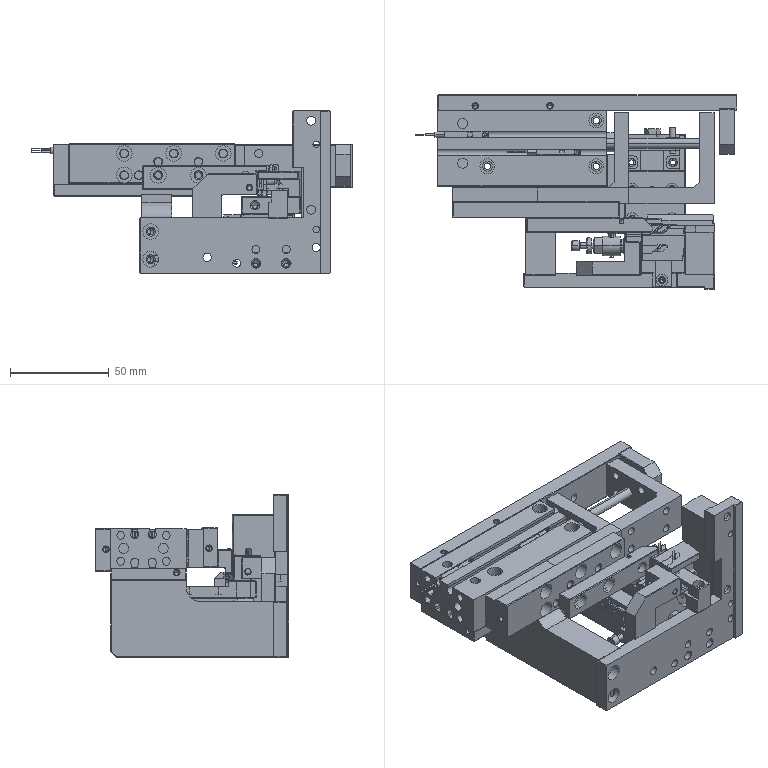Part | NX | 29 solids | 2576 faces | box 162.5 x 98 x 82 mm | volume 328768 mm3 | plane 1297 | cylinder 863 | cone 288 | torus 58 | spline 58 | sphere 12 | commonest cylinder face diameters 4 x128 0.2 x96 3 x56 4.5 x52 3.3 x50 2.5 x48